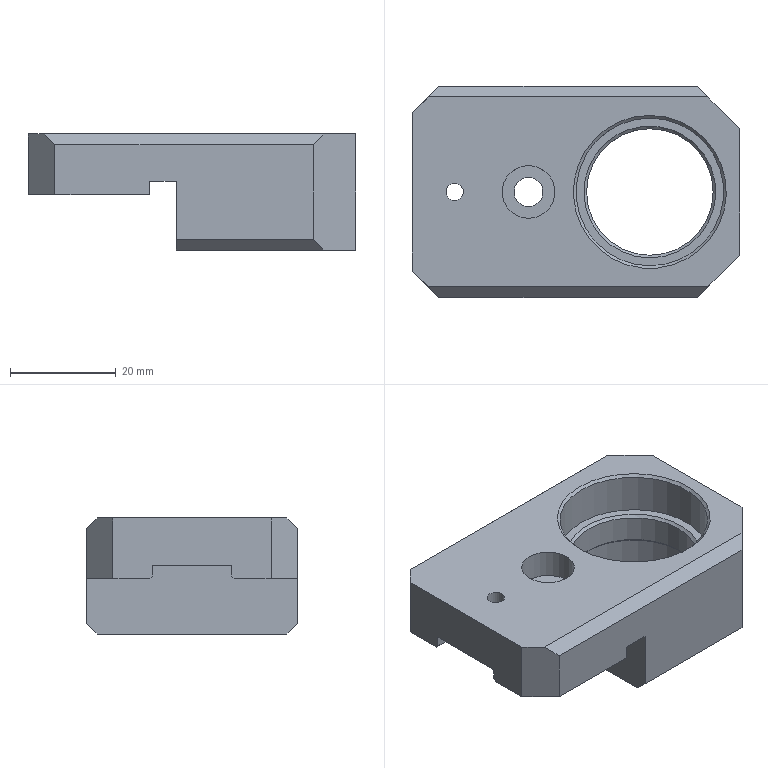NC program | NX | posted with a generic post | part box 62 x 40 x 22 mm
Whole program:
N10 G17 G21 G94 G90
(FLOOR_WALL , TOOL : D63)
N12 T01 M6
N14 G54
N16 G17 G0 G90 X-67.5 Y0. S6500 M3
N18 G43 Z30. H1
N20 Z3.
N22 G94 G1 Z0. F1500.
N24 X-64.5
N26 X64.5
N28 X67.5
N30 Z3.
N32 G0 Z30.
N34 M5
(DRILLING , TOOL : D8A45)
N36 T06 M6
N38 G54
N40 G17 G0 G90 X-9. Y0. S3500 M3
N42 G43 Z30. H6
N44 G94 G81 G98 Z-1. F250. R3.
N46 X14.
N48 X-23.
N50 G80
N52 G0 X-23. Y0. Z30.
N54 M5
(DRILLING_COPY , TOOL : 3.3ZT)
N56 T12 M6
N58 G54
N60 G17 G0 G90 X-23. Y0. S1500 M3
N62 G43 Z30. H12
N64 G94 G83 G98 Z-11.491 F150. Q2. R3.
N66 G80
N68 G0 X-23. Y0. Z30.
N70 M5
(DRILLING_1 , TOOL : 5.5ZT)
N72 T22 M6
N74 G54
N76 G17 G0 G90 X-9. Y0. S2000 M3
N78 G43 Z30. H22
N80 G94 G83 G98 Z-12.152 F200. Q3. R3.
N82 G80
N84 G0 X-9. Y0. Z30.
N86 M5
(ZLEVEL_PROFILE , TOOL : D10)
N88 T04 M6
N90 G54
N92 G17 G0 G90 X36.1 Y-8.145 S7000 M3
N94 G43 Z30. H4
N96 Z1.5
N98 G94 G1 Y-12. Z1.298 F1000.
N100 Y-12.554 Z1.269
N102 X35.74 Y-13.963 Z1.193
N104 X34.998 Y-15.215 Z1.116
N106 X26.215 Y-23.998 Z0.465
N108 X24.963 Y-24.74 Z0.389
N110 X23.554 Y-25.1 Z0.313
N112 X-1.5 Z-1.
N114 X-26. F3000.
N116 G2 X-29.606 Y-23.606 R5.1
N118 G1 X-34.606 Y-18.606
N120 G2 X-36.1 Y-15. R5.1
N122 G1 Y15.
N124 G2 X-34.606 Y18.606 R5.1
N126 G1 X-29.606 Y23.606
N128 G2 X-26. Y25.1 R5.1
N130 G1 X23.
N132 G2 X26.606 Y23.606 R5.1
N134 G1 X34.606 Y15.606
N136 G2 X36.1 Y12. R5.1
N138 G1 Y-12.
N140 G2 X34.606 Y-15.606 R5.1
N142 G1 X26.606 Y-23.606
N144 G2 X23. Y-25.1 R5.1
N146 G1 X-1.5
N148 X-25.5 Z-1.419
N150 X-25.887 Z-1.426
N152 X-26.274 Y-25.093 Z-1.432
N154 X-26.659 Y-25.057 Z-1.439
N156 X-27.041 Y-24.993 Z-1.446
N158 X-27.416 Y-24.899 Z-1.453
N160 X-27.784 Y-24.778 Z-1.459
N162 X-28.141 Y-24.629 Z-1.466
N164 X-28.486 Y-24.453 Z-1.473
N166 X-28.816 Y-24.252 Z-1.48
N168 X-29.131 Y-24.026 Z-1.486
N170 X-29.427 Y-23.777 Z-1.493
N172 X-29.705 Y-23.508 Z-1.5
N174 X-34.358 Y-18.854 Z-1.615
N176 X-34.632 Y-18.581 Z-1.622
N178 X-34.893 Y-18.295 Z-1.628
N180 X-35.131 Y-17.99 Z-1.635
N182 X-35.346 Y-17.668 Z-1.642
N184 X-35.536 Y-17.331 Z-1.649
N186 X-35.7 Y-16.98 Z-1.655
N188 X-35.836 Y-16.618 Z-1.662
N190 X-35.945 Y-16.247 Z-1.669
N192 X-36.026 Y-15.868 Z-1.676
N194 X-36.077 Y-15.485 Z-1.682
N196 X-36.099 Y-15.099 Z-1.689
N198 X-36.1 Y-14.711 Z-1.696
N200 Y-14.324 Z-1.703
N202 Y2.708 Z-2.
N204 Y15.
N206 G2 X-34.606 Y18.606 R5.1
N208 G1 X-29.606 Y23.606
N210 G2 X-26. Y25.1 R5.1
N212 G1 X23.
N214 G2 X26.606 Y23.606 R5.1
N216 G1 X34.606 Y15.606
N218 G2 X36.1 Y12. R5.1
N220 G1 Y-12.
N222 G2 X34.606 Y-15.606 R5.1
N224 G1 X26.606 Y-23.606
N226 G2 X23. Y-25.1 R5.1
N228 G1 X-1.5
N230 X-25.5 Z-2.419
N232 X-25.887 Z-2.426
N234 X-26.274 Y-25.093 Z-2.432
N236 X-26.659 Y-25.057 Z-2.439
N238 X-27.041 Y-24.993 Z-2.446
N240 X-27.416 Y-24.899 Z-2.453
N242 X-27.784 Y-24.778 Z-2.459
N244 X-28.141 Y-24.629 Z-2.466
N246 X-28.486 Y-24.453 Z-2.473
N248 X-28.816 Y-24.252 Z-2.48
N250 X-29.131 Y-24.026 Z-2.486
N252 X-29.427 Y-23.777 Z-2.493
N254 X-29.705 Y-23.508 Z-2.5
N256 X-34.358 Y-18.854 Z-2.615
N258 X-34.632 Y-18.581 Z-2.622
N260 X-34.893 Y-18.295 Z-2.628
N262 X-35.131 Y-17.99 Z-2.635
N264 X-35.346 Y-17.668 Z-2.642
N266 X-35.536 Y-17.331 Z-2.649
N268 X-35.7 Y-16.98 Z-2.655
N270 X-35.836 Y-16.618 Z-2.662
N272 X-35.945 Y-16.247 Z-2.669
N274 X-36.026 Y-15.868 Z-2.676
N276 X-36.077 Y-15.485 Z-2.682
N278 X-36.099 Y-15.099 Z-2.689
N280 X-36.1 Y-14.711 Z-2.696
N282 Y-14.324 Z-2.703
N284 Y2.708 Z-3.
N286 Y15.
N288 G2 X-34.606 Y18.606 R5.1
N290 G1 X-29.606 Y23.606
N292 G2 X-26. Y25.1 R5.1
N294 G1 X23.
N296 G2 X26.606 Y23.606 R5.1
N298 G1 X34.606 Y15.606
N300 G2 X36.1 Y12. R5.1
N302 G1 Y-12.
N304 G2 X34.606 Y-15.606 R5.1
N306 G1 X26.606 Y-23.606
N308 G2 X23. Y-25.1 R5.1
N310 G1 X-1.5
N312 X-25.5 Z-3.419
N314 X-25.887 Z-3.426
N316 X-26.274 Y-25.093 Z-3.432
N318 X-26.659 Y-25.057 Z-3.439
N320 X-27.041 Y-24.993 Z-3.446
N322 X-27.416 Y-24.899 Z-3.453
N324 X-27.784 Y-24.778 Z-3.459
N326 X-28.141 Y-24.629 Z-3.466
N328 X-28.486 Y-24.453 Z-3.473
N330 X-28.816 Y-24.252 Z-3.48
N332 X-29.131 Y-24.026 Z-3.486
N334 X-29.427 Y-23.777 Z-3.493
N336 X-29.705 Y-23.508 Z-3.5
N338 X-34.358 Y-18.854 Z-3.615
N340 X-34.632 Y-18.581 Z-3.622
N342 X-34.893 Y-18.295 Z-3.628
N344 X-35.131 Y-17.99 Z-3.635
N346 X-35.346 Y-17.668 Z-3.642
N348 X-35.536 Y-17.331 Z-3.649
N350 X-35.7 Y-16.98 Z-3.655
N352 X-35.836 Y-16.618 Z-3.662
N354 X-35.945 Y-16.247 Z-3.669
N356 X-36.026 Y-15.868 Z-3.676
N358 X-36.077 Y-15.485 Z-3.682
N360 X-36.099 Y-15.099 Z-3.689
N362 X-36.1 Y-14.711 Z-3.696
N364 Y-14.324 Z-3.703
N366 Y2.708 Z-4.
N368 Y15.
N370 G2 X-34.606 Y18.606 R5.1
N372 G1 X-29.606 Y23.606
N374 G2 X-26. Y25.1 R5.1
N376 G1 X23.
N378 G2 X26.606 Y23.606 R5.1
N380 G1 X34.606 Y15.606
N382 G2 X36.1 Y12. R5.1
N384 G1 Y-12.
N386 G2 X34.606 Y-15.606 R5.1
N388 G1 X26.606 Y-23.606
N390 G2 X23. Y-25.1 R5.1
N392 G1 X-1.5
N394 X-25.5 Z-4.419
N396 X-25.887 Z-4.426
N398 X-26.274 Y-25.093 Z-4.432
N400 X-26.659 Y-25.057 Z-4.439
N402 X-27.041 Y-24.993 Z-4.446
N404 X-27.416 Y-24.899 Z-4.453
N406 X-27.784 Y-24.778 Z-4.459
N408 X-28.141 Y-24.629 Z-4.466
N410 X-28.486 Y-24.453 Z-4.473
N412 X-28.816 Y-24.252 Z-4.48
N414 X-29.131 Y-24.026 Z-4.486
N416 X-29.427 Y-23.777 Z-4.493
N418 X-29.705 Y-23.508 Z-4.5
N420 X-34.358 Y-18.854 Z-4.615
N422 X-34.632 Y-18.581 Z-4.622
N424 X-34.893 Y-18.295 Z-4.628
N426 X-35.131 Y-17.99 Z-4.635
N428 X-35.346 Y-17.668 Z-4.642
N430 X-35.536 Y-17.331 Z-4.649
N432 X-35.7 Y-16.98 Z-4.655
N434 X-35.836 Y-16.618 Z-4.662
N436 X-35.945 Y-16.247 Z-4.669
N438 X-36.026 Y-15.868 Z-4.676
N440 X-36.077 Y-15.485 Z-4.682
N442 X-36.099 Y-15.099 Z-4.689
N444 X-36.1 Y-14.711 Z-4.696
N446 Y-14.324 Z-4.703
N448 Y2.708 Z-5.
N450 Y15.
N452 G2 X-34.606 Y18.606 R5.1
N454 G1 X-29.606 Y23.606
N456 G2 X-26. Y25.1 R5.1
N458 G1 X23.
N460 G2 X26.606 Y23.606 R5.1
N462 G1 X34.606 Y15.606
N464 G2 X36.1 Y12. R5.1
N466 G1 Y-12.
N468 G2 X34.606 Y-15.606 R5.1
N470 G1 X26.606 Y-23.606
N472 G2 X23. Y-25.1 R5.1
N474 G1 X-1.5
N476 X-25.5 Z-5.419
N478 X-25.887 Z-5.426
N480 X-26.274 Y-25.093 Z-5.432
N482 X-26.659 Y-25.057 Z-5.439
N484 X-27.041 Y-24.993 Z-5.446
N486 X-27.416 Y-24.899 Z-5.453
N488 X-27.784 Y-24.778 Z-5.459
N490 X-28.141 Y-24.629 Z-5.466
N492 X-28.486 Y-24.453 Z-5.473
N494 X-28.816 Y-24.252 Z-5.48
N496 X-29.131 Y-24.026 Z-5.486
N498 X-29.427 Y-23.777 Z-5.493
N500 X-29.705 Y-23.508 Z-5.5
N502 X-34.358 Y-18.854 Z-5.615
N504 X-34.632 Y-18.581 Z-5.622
N506 X-34.893 Y-18.295 Z-5.628
N508 X-35.131 Y-17.99 Z-5.635
N510 X-35.346 Y-17.668 Z-5.642
N512 X-35.536 Y-17.331 Z-5.649
N514 X-35.7 Y-16.98 Z-5.655
N516 X-35.836 Y-16.618 Z-5.662
N518 X-35.945 Y-16.247 Z-5.669
N520 X-36.026 Y-15.868 Z-5.676
N522 X-36.077 Y-15.485 Z-5.682
N524 X-36.099 Y-15.099 Z-5.689
N526 X-36.1 Y-14.711 Z-5.696
N528 Y-14.324 Z-5.703
N530 Y2.708 Z-6.
N532 Y15.
N534 G2 X-34.606 Y18.606 R5.1
N536 G1 X-29.606 Y23.606
N538 G2 X-26. Y25.1 R5.1
N540 G1 X23.
N542 G2 X26.606 Y23.606 R5.1
N544 G1 X34.606 Y15.606
N546 G2 X36.1 Y12. R5.1
N548 G1 Y-12.
N550 G2 X34.606 Y-15.606 R5.1
N552 G1 X26.606 Y-23.606
N554 G2 X23. Y-25.1 R5.1
N556 G1 X-1.5
N558 X-25.5 Z-6.419
N560 X-25.887 Z-6.426
N562 X-26.274 Y-25.093 Z-6.432
N564 X-26.659 Y-25.057 Z-6.439
N566 X-27.041 Y-24.993 Z-6.446
N568 X-27.416 Y-24.899 Z-6.453
N570 X-27.784 Y-24.778 Z-6.459
N572 X-28.141 Y-24.629 Z-6.466
N574 X-28.486 Y-24.453 Z-6.473
N576 X-28.816 Y-24.252 Z-6.48
N578 X-29.131 Y-24.026 Z-6.486
N580 X-29.427 Y-23.777 Z-6.493
N582 X-29.705 Y-23.508 Z-6.5
N584 X-34.358 Y-18.854 Z-6.615
N586 X-34.632 Y-18.581 Z-6.622
N588 X-34.893 Y-18.295 Z-6.628
N590 X-35.131 Y-17.99 Z-6.635
N592 X-35.346 Y-17.668 Z-6.642
N594 X-35.536 Y-17.331 Z-6.649
N596 X-35.7 Y-16.98 Z-6.655
N598 X-35.836 Y-16.618 Z-6.662
N600 X-35.945 Y-16.247 Z-6.669
N602 X-36.026 Y-15.868 Z-6.676
N604 X-36.077 Y-15.485 Z-6.682
N606 X-36.099 Y-15.099 Z-6.689
N608 X-36.1 Y-14.711 Z-6.696
N610 Y-14.324 Z-6.703
N612 Y2.708 Z-7.
N614 Y15.
N616 G2 X-34.606 Y18.606 R5.1
N618 G1 X-29.606 Y23.606
N620 G2 X-26. Y25.1 R5.1
N622 G1 X23.
N624 G2 X26.606 Y23.606 R5.1
N626 G1 X34.606 Y15.606
N628 G2 X36.1 Y12. R5.1
N630 G1 Y-12.
N632 G2 X34.606 Y-15.606 R5.1
N634 G1 X26.606 Y-23.606
N636 G2 X23. Y-25.1 R5.1
N638 G1 X-1.5
N640 X-25.5 Z-7.419
N642 X-25.887 Z-7.426
N644 X-26.274 Y-25.093 Z-7.432
N646 X-26.659 Y-25.057 Z-7.439
N648 X-27.041 Y-24.993 Z-7.446
N650 X-27.416 Y-24.899 Z-7.453
N652 X-27.784 Y-24.778 Z-7.459
N654 X-28.141 Y-24.629 Z-7.466
N656 X-28.486 Y-24.453 Z-7.473
N658 X-28.816 Y-24.252 Z-7.48
N660 X-29.131 Y-24.026 Z-7.486
N662 X-29.427 Y-23.777 Z-7.493
N664 X-29.705 Y-23.508 Z-7.5
N666 X-34.358 Y-18.854 Z-7.615
N668 X-34.632 Y-18.581 Z-7.622
N670 X-34.893 Y-18.295 Z-7.628
N672 X-35.131 Y-17.99 Z-7.635
N674 X-35.346 Y-17.668 Z-7.642
N676 X-35.536 Y-17.331 Z-7.649
N678 X-35.7 Y-16.98 Z-7.655
N680 X-35.836 Y-16.618 Z-7.662
N682 X-35.945 Y-16.247 Z-7.669
N684 X-36.026 Y-15.868 Z-7.676
N686 X-36.077 Y-15.485 Z-7.682
N688 X-36.099 Y-15.099 Z-7.689
N690 X-36.1 Y-14.711 Z-7.696
N692 Y-14.324 Z-7.703
N694 Y2.708 Z-8.
N696 Y15.
N698 G2 X-34.606 Y18.606 R5.1
N700 G1 X-29.606 Y23.606
N702 G2 X-26. Y25.1 R5.1
N704 G1 X23.
N706 G2 X26.606 Y23.606 R5.1
N708 G1 X34.606 Y15.606
N710 G2 X36.1 Y12. R5.1
N712 G1 Y-12.
N714 G2 X34.606 Y-15.606 R5.1
N716 G1 X26.606 Y-23.606
N718 G2 X23. Y-25.1 R5.1
N720 G1 X-1.5
N722 X-25.5 Z-8.419
N724 X-25.887 Z-8.426
N726 X-26.274 Y-25.093 Z-8.432
N728 X-26.659 Y-25.057 Z-8.439
N730 X-27.041 Y-24.993 Z-8.446
N732 X-27.416 Y-24.899 Z-8.453
N734 X-27.784 Y-24.778 Z-8.459
N736 X-28.141 Y-24.629 Z-8.466
N738 X-28.486 Y-24.453 Z-8.473
N740 X-28.816 Y-24.252 Z-8.48
N742 X-29.131 Y-24.026 Z-8.486
N744 X-29.427 Y-23.777 Z-8.493
N746 X-29.705 Y-23.508 Z-8.5
N748 X-34.358 Y-18.854 Z-8.615
N750 X-34.632 Y-18.581 Z-8.622
N752 X-34.893 Y-18.295 Z-8.628
N754 X-35.131 Y-17.99 Z-8.635
N756 X-35.346 Y-17.668 Z-8.642
N758 X-35.536 Y-17.331 Z-8.649
N760 X-35.7 Y-16.98 Z-8.655
N762 X-35.836 Y-16.618 Z-8.662
N764 X-35.945 Y-16.247 Z-8.669
N766 X-36.026 Y-15.868 Z-8.676
N768 X-36.077 Y-15.485 Z-8.682
N770 X-36.099 Y-15.099 Z-8.689
N772 X-36.1 Y-14.711 Z-8.696
N774 Y-14.324 Z-8.703
N776 Y2.708 Z-9.
N778 Y15.
N780 G2 X-34.606 Y18.606 R5.1
N782 G1 X-29.606 Y23.606
N784 G2 X-26. Y25.1 R5.1
N786 G1 X23.
N788 G2 X26.606 Y23.606 R5.1
N790 G1 X34.606 Y15.606
N792 G2 X36.1 Y12. R5.1
N794 G1 Y-12.
N796 G2 X34.606 Y-15.606 R5.1
N798 G1 X26.606 Y-23.606
N800 G2 X23. Y-25.1 R5.1
N802 G1 X-1.5
N804 X-25.5 Z-9.419
N806 X-25.887 Z-9.426
N808 X-26.274 Y-25.093 Z-9.432
N810 X-26.659 Y-25.057 Z-9.439
N812 X-27.041 Y-24.993 Z-9.446
N814 X-27.416 Y-24.899 Z-9.453
N816 X-27.784 Y-24.778 Z-9.459
N818 X-28.141 Y-24.629 Z-9.466
N820 X-28.486 Y-24.453 Z-9.473
N822 X-28.816 Y-24.252 Z-9.48
N824 X-29.131 Y-24.026 Z-9.486
N826 X-29.427 Y-23.777 Z-9.493
N828 X-29.705 Y-23.508 Z-9.5
N830 X-34.358 Y-18.854 Z-9.615
N832 X-34.632 Y-18.581 Z-9.622
N834 X-34.893 Y-18.295 Z-9.628
N836 X-35.131 Y-17.99 Z-9.635
N838 X-35.346 Y-17.668 Z-9.642
N840 X-35.536 Y-17.331 Z-9.649
N842 X-35.7 Y-16.98 Z-9.655
N844 X-35.836 Y-16.618 Z-9.662
N846 X-35.945 Y-16.247 Z-9.669
N848 X-36.026 Y-15.868 Z-9.676
N850 X-36.077 Y-15.485 Z-9.682
N852 X-36.099 Y-15.099 Z-9.689
N854 X-36.1 Y-14.711 Z-9.696
N856 Y-14.324 Z-9.703
N858 Y2.708 Z-10.
N860 Y15.
N862 G2 X-34.606 Y18.606 R5.1
N864 G1 X-29.606 Y23.606
N866 G2 X-26. Y25.1 R5.1
N868 G1 X23.
N870 G2 X26.606 Y23.606 R5.1
N872 G1 X34.606 Y15.606
N874 G2 X36.1 Y12. R5.1
N876 G1 Y-12.
N878 G2 X34.606 Y-15.606 R5.1
N880 G1 X26.606 Y-23.606
N882 G2 X23. Y-25.1 R5.1
N884 G1 X-1.5
N886 X-25.5 Z-10.419
N888 X-25.887 Z-10.426
N890 X-26.274 Y-25.093 Z-10.432
N892 X-26.659 Y-25.057 Z-10.439
N894 X-27.041 Y-24.993 Z-10.446
N896 X-27.416 Y-24.899 Z-10.453
N898 X-27.784 Y-24.778 Z-10.459
N900 X-28.141 Y-24.629 Z-10.466
N902 X-28.486 Y-24.453 Z-10.473
N904 X-28.816 Y-24.252 Z-10.48
N906 X-29.131 Y-24.026 Z-10.486
N908 X-29.427 Y-23.777 Z-10.493
N910 X-29.705 Y-23.508 Z-10.5
N912 X-34.358 Y-18.854 Z-10.615
N914 X-34.632 Y-18.581 Z-10.622
N916 X-34.893 Y-18.295 Z-10.628
N918 X-35.131 Y-17.99 Z-10.635
N920 X-35.346 Y-17.668 Z-10.642
N922 X-35.536 Y-17.331 Z-10.649
N924 X-35.7 Y-16.98 Z-10.655
N926 X-35.836 Y-16.618 Z-10.662
N928 X-35.945 Y-16.247 Z-10.669
N930 X-36.026 Y-15.868 Z-10.676
N932 X-36.077 Y-15.485 Z-10.682
N934 X-36.099 Y-15.099 Z-10.689
N936 X-36.1 Y-14.711 Z-10.696
N938 Y-14.324 Z-10.703
N940 Y2.708 Z-11.
N942 Y15.
N944 G2 X-34.606 Y18.606 R5.1
N946 G1 X-29.606 Y23.606
N948 G2 X-26. Y25.1 R5.1
N950 G1 X23.
N952 G2 X26.606 Y23.606 R5.1
N954 G1 X34.606 Y15.606
N956 G2 X36.1 Y12. R5.1
N958 G1 Y-12.
N960 G2 X34.606 Y-15.606 R5.1
N962 G1 X26.606 Y-23.606
N964 G2 X23. Y-25.1 R5.1
N966 G1 X-1.5
N968 X-25.5 Z-11.419
N970 X-25.887 Z-11.426
N972 X-26.274 Y-25.093 Z-11.432
N974 X-26.659 Y-25.057 Z-11.439
N976 X-27.041 Y-24.993 Z-11.446
N978 X-27.416 Y-24.899 Z-11.453
N980 X-27.784 Y-24.778 Z-11.459
N982 X-28.141 Y-24.629 Z-11.466
N984 X-28.486 Y-24.453 Z-11.473
N986 X-28.816 Y-24.252 Z-11.48
N988 X-29.131 Y-24.026 Z-11.486
N990 X-29.427 Y-23.777 Z-11.493
N992 X-29.705 Y-23.508 Z-11.5
N994 X-34.358 Y-18.854 Z-11.615
N996 X-34.632 Y-18.581 Z-11.622
N998 X-34.893 Y-18.295 Z-11.628
N1000 X-35.131 Y-17.99 Z-11.635
N1002 X-35.346 Y-17.668 Z-11.642
N1004 X-35.536 Y-17.331 Z-11.649
N1006 X-35.7 Y-16.98 Z-11.655
N1008 X-35.836 Y-16.618 Z-11.662
N1010 X-35.945 Y-16.247 Z-11.669
N1012 X-36.026 Y-15.868 Z-11.676
N1014 X-36.077 Y-15.485 Z-11.682
N1016 X-36.099 Y-15.099 Z-11.689
N1018 X-36.1 Y-14.711 Z-11.696
N1020 Y-14.324 Z-11.703
N1022 Y2.708 Z-12.
N1024 Y15.
N1026 G2 X-34.606 Y18.606 R5.1
N1028 G1 X-29.606 Y23.606
N1030 G2 X-26. Y25.1 R5.1
N1032 G1 X23.
N1034 G2 X26.606 Y23.606 R5.1
N1036 G1 X34.606 Y15.606
N1038 G2 X36.1 Y12. R5.1
N1040 G1 Y-12.
N1042 G2 X34.606 Y-15.606 R5.1
N1044 G1 X26.606 Y-23.606
N1046 G2 X23. Y-25.1 R5.1
N1048 G1 X-1.5
N1050 X-25.5 Z-12.419
N1052 X-25.887 Z-12.426
N1054 X-26.274 Y-25.093 Z-12.432
N1056 X-26.659 Y-25.057 Z-12.439
N1058 X-27.041 Y-24.993 Z-12.446
N1060 X-27.416 Y-24.899 Z-12.453
N1062 X-27.784 Y-24.778 Z-12.459
N1064 X-28.141 Y-24.629 Z-12.466
N1066 X-28.486 Y-24.453 Z-12.473
N1068 X-28.816 Y-24.252 Z-12.48
N1070 X-29.131 Y-24.026 Z-12.486
N1072 X-29.427 Y-23.777 Z-12.493
N1074 X-29.705 Y-23.508 Z-12.5
N1076 X-34.358 Y-18.854 Z-12.615
N1078 X-34.632 Y-18.581 Z-12.622
N1080 X-34.893 Y-18.295 Z-12.628
N1082 X-35.131 Y-17.99 Z-12.635
N1084 X-35.346 Y-17.668 Z-12.642
N1086 X-35.536 Y-17.331 Z-12.649
N1088 X-35.7 Y-16.98 Z-12.655
N1090 X-35.836 Y-16.618 Z-12.662
N1092 X-35.945 Y-16.247 Z-12.669
N1094 X-36.026 Y-15.868 Z-12.676
N1096 X-36.077 Y-15.485 Z-12.682
N1098 X-36.099 Y-15.099 Z-12.689
N1100 X-36.1 Y-14.711 Z-12.696
N1102 Y-14.324 Z-12.703
N1104 Y2.708 Z-13.
N1106 Y15.
N1108 G2 X-34.606 Y18.606 R5.1
N1110 G1 X-29.606 Y23.606
N1112 G2 X-26. Y25.1 R5.1
N1114 G1 X23.
N1116 G2 X26.606 Y23.606 R5.1
N1118 G1 X34.606 Y15.606
N1120 G2 X36.1 Y12. R5.1
N1122 G1 Y-12.
N1124 G2 X34.606 Y-15.606 R5.1
N1126 G1 X26.606 Y-23.606
N1128 G2 X23. Y-25.1 R5.1
N1130 G1 X-1.5
N1132 X-25.5 Z-13.419
N1134 X-25.887 Z-13.426
N1136 X-26.274 Y-25.093 Z-13.432
N1138 X-26.659 Y-25.057 Z-13.439
N1140 X-27.041 Y-24.993 Z-13.446
N1142 X-27.416 Y-24.899 Z-13.453
N1144 X-27.784 Y-24.778 Z-13.459
N1146 X-28.141 Y-24.629 Z-13.466
N1148 X-28.486 Y-24.453 Z-13.473
N1150 X-28.816 Y-24.252 Z-13.48
N1152 X-29.131 Y-24.026 Z-13.486
N1154 X-29.427 Y-23.777 Z-13.493
N1156 X-29.705 Y-23.508 Z-13.5
N1158 X-34.358 Y-18.854 Z-13.615
N1160 X-34.632 Y-18.581 Z-13.622
N1162 X-34.893 Y-18.295 Z-13.628
N1164 X-35.131 Y-17.99 Z-13.635
N1166 X-35.346 Y-17.668 Z-13.642
N1168 X-35.536 Y-17.331 Z-13.649
N1170 X-35.7 Y-16.98 Z-13.655
N1172 X-35.836 Y-16.618 Z-13.662
N1174 X-35.945 Y-16.247 Z-13.669
N1176 X-36.026 Y-15.868 Z-13.676
N1178 X-36.077 Y-15.485 Z-13.682
N1180 X-36.099 Y-15.099 Z-13.689
N1182 X-36.1 Y-14.711 Z-13.696
N1184 Y-14.324 Z-13.703
N1186 Y2.708 Z-14.
N1188 Y15.
N1190 G2 X-34.606 Y18.606 R5.1
N1192 G1 X-29.606 Y23.606
N1194 G2 X-26. Y25.1 R5.1
N1196 G1 X23.
N1198 G2 X26.606 Y23.606 R5.1
N1200 G1 X34.606 Y15.606
N1202 G2 X36.1 Y12. R5.1
N1204 G1 Y-12.
N1206 G2 X34.606 Y-15.606 R5.1
N1208 G1 X26.606 Y-23.606
N1210 G2 X23. Y-25.1 R5.1
N1212 G1 X-1.5
N1214 X-25.5 Z-14.419
N1216 X-25.887 Z-14.426
N1218 X-26.274 Y-25.093 Z-14.432
N1220 X-26.659 Y-25.057 Z-14.439
N1222 X-27.041 Y-24.993 Z-14.446
N1224 X-27.416 Y-24.899 Z-14.453
N1226 X-27.784 Y-24.778 Z-14.459
N1228 X-28.141 Y-24.629 Z-14.466
N1230 X-28.486 Y-24.453 Z-14.473
N1232 X-28.816 Y-24.252 Z-14.48
N1234 X-29.131 Y-24.026 Z-14.486
N1236 X-29.427 Y-23.777 Z-14.493
N1238 X-29.705 Y-23.508 Z-14.5
N1240 X-34.358 Y-18.854 Z-14.615
N1242 X-34.632 Y-18.581 Z-14.622
N1244 X-34.893 Y-18.295 Z-14.628
N1246 X-35.131 Y-17.99 Z-14.635
N1248 X-35.346 Y-17.668 Z-14.642
N1250 X-35.536 Y-17.331 Z-14.649
N1252 X-35.7 Y-16.98 Z-14.655
N1254 X-35.836 Y-16.618 Z-14.662
N1256 X-35.945 Y-16.247 Z-14.669
N1258 X-36.026 Y-15.868 Z-14.676
N1260 X-36.077 Y-15.485 Z-14.682
N1262 X-36.099 Y-15.099 Z-14.689
N1264 X-36.1 Y-14.711 Z-14.696
N1266 Y-14.324 Z-14.703
N1268 Y2.708 Z-15.
N1270 Y15.
N1272 G2 X-34.606 Y18.606 R5.1
N1274 G1 X-29.606 Y23.606
N1276 G2 X-26. Y25.1 R5.1
N1278 G1 X23.
N1280 G2 X26.606 Y23.606 R5.1
N1282 G1 X34.606 Y15.606
N1284 G2 X36.1 Y12. R5.1
N1286 G1 Y-12.
N1288 G2 X34.606 Y-15.606 R5.1
N1290 G1 X26.606 Y-23.606
N1292 G2 X23. Y-25.1 R5.1
N1294 G1 X-1.5
N1296 X-25.5 Z-15.419
N1298 X-25.887 Z-15.426
N1300 X-26.274 Y-25.093 Z-15.432
N1302 X-26.659 Y-25.057 Z-15.439
N1304 X-27.041 Y-24.993 Z-15.446
N1306 X-27.416 Y-24.899 Z-15.453
N1308 X-27.784 Y-24.778 Z-15.459
N1310 X-28.141 Y-24.629 Z-15.466
N1312 X-28.486 Y-24.453 Z-15.473
N1314 X-28.816 Y-24.252 Z-15.48
N1316 X-29.131 Y-24.026 Z-15.486
N1318 X-29.427 Y-23.777 Z-15.493
N1320 X-29.705 Y-23.508 Z-15.5
N1322 X-34.358 Y-18.854 Z-15.615
N1324 X-34.632 Y-18.581 Z-15.622
N1326 X-34.893 Y-18.295 Z-15.628
N1328 X-35.131 Y-17.99 Z-15.635
N1330 X-35.346 Y-17.668 Z-15.642
N1332 X-35.536 Y-17.331 Z-15.649
N1334 X-35.7 Y-16.98 Z-15.655
N1336 X-35.836 Y-16.618 Z-15.662
N1338 X-35.945 Y-16.247 Z-15.669
N1340 X-36.026 Y-15.868 Z-15.676
N1342 X-36.077 Y-15.485 Z-15.682
N1344 X-36.099 Y-15.099 Z-15.689
N1346 X-36.1 Y-14.711 Z-15.696
N1348 Y-14.324 Z-15.703
N1350 Y2.708 Z-16.
N1352 Y15.
N1354 G2 X-34.606 Y18.606 R5.1
N1356 G1 X-29.606 Y23.606
N1358 G2 X-26. Y25.1 R5.1
N1360 G1 X23.
N1362 G2 X26.606 Y23.606 R5.1
N1364 G1 X34.606 Y15.606
N1366 G2 X36.1 Y12. R5.1
N1368 G1 Y-12.
N1370 G2 X34.606 Y-15.606 R5.1
N1372 G1 X26.606 Y-23.606
N1374 G2 X23. Y-25.1 R5.1
N1376 G1 X-1.5
N1378 X-25.5 Z-16.419
N1380 X-25.887 Z-16.426
N1382 X-26.274 Y-25.093 Z-16.432
N1384 X-26.659 Y-25.057 Z-16.439
N1386 X-27.041 Y-24.993 Z-16.446
N1388 X-27.416 Y-24.899 Z-16.453
N1390 X-27.784 Y-24.778 Z-16.459
N1392 X-28.141 Y-24.629 Z-16.466
N1394 X-28.486 Y-24.453 Z-16.473
N1396 X-28.816 Y-24.252 Z-16.48
N1398 X-29.131 Y-24.026 Z-16.486
N1400 X-29.427 Y-23.777 Z-16.493
N1402 X-29.705 Y-23.508 Z-16.5
N1404 X-34.358 Y-18.854 Z-16.615
N1406 X-34.632 Y-18.581 Z-16.622
N1408 X-34.893 Y-18.295 Z-16.628
N1410 X-35.131 Y-17.99 Z-16.635
N1412 X-35.346 Y-17.668 Z-16.642
N1414 X-35.536 Y-17.331 Z-16.649
N1416 X-35.7 Y-16.98 Z-16.655
N1418 X-35.836 Y-16.618 Z-16.662
N1420 X-35.945 Y-16.247 Z-16.669
N1422 X-36.026 Y-15.868 Z-16.676
N1424 X-36.077 Y-15.485 Z-16.682
N1426 X-36.099 Y-15.099 Z-16.689
N1428 X-36.1 Y-14.711 Z-16.696
N1430 Y-14.324 Z-16.703
N1432 Y2.708 Z-17.
N1434 Y15.
N1436 G2 X-34.606 Y18.606 R5.1
N1438 G1 X-29.606 Y23.606
N1440 G2 X-26. Y25.1 R5.1
N1442 G1 X23.
N1444 G2 X26.606 Y23.606 R5.1
N1446 G1 X34.606 Y15.606
N1448 G2 X36.1 Y12. R5.1
N1450 G1 Y-12.
N1452 G2 X34.606 Y-15.606 R5.1
N1454 G1 X26.606 Y-23.606
N1456 G2 X23. Y-25.1 R5.1
N1458 G1 X-1.5
N1460 X-25.5 Z-17.419
N1462 X-25.887 Z-17.426
N1464 X-26.274 Y-25.093 Z-17.432
N1466 X-26.659 Y-25.057 Z-17.439
N1468 X-27.041 Y-24.993 Z-17.446
N1470 X-27.416 Y-24.899 Z-17.453
N1472 X-27.784 Y-24.778 Z-17.459
N1474 X-28.141 Y-24.629 Z-17.466
N1476 X-28.486 Y-24.453 Z-17.473
N1478 X-28.816 Y-24.252 Z-17.48
N1480 X-29.131 Y-24.026 Z-17.486
N1482 X-29.427 Y-23.777 Z-17.493
N1484 X-29.705 Y-23.508 Z-17.5
N1486 X-34.358 Y-18.854 Z-17.615
N1488 X-34.632 Y-18.581 Z-17.622
N1490 X-34.893 Y-18.295 Z-17.628
N1492 X-35.131 Y-17.99 Z-17.635
N1494 X-35.346 Y-17.668 Z-17.642
N1496 X-35.536 Y-17.331 Z-17.649
N1498 X-35.7 Y-16.98 Z-17.655
N1500 X-35.836 Y-16.618 Z-17.662
N1502 X-35.945 Y-16.247 Z-17.669
N1504 X-36.026 Y-15.868 Z-17.676
N1506 X-36.077 Y-15.485 Z-17.682
N1508 X-36.099 Y-15.099 Z-17.689
N1510 X-36.1 Y-14.711 Z-17.696
N1512 Y-14.324 Z-17.703
N1514 Y2.708 Z-18.
N1516 Y15.
N1518 G2 X-34.606 Y18.606 R5.1
N1520 G1 X-29.606 Y23.606
N1522 G2 X-26. Y25.1 R5.1
N1524 G1 X23.
N1526 G2 X26.606 Y23.606 R5.1
N1528 G1 X34.606 Y15.606
N1530 G2 X36.1 Y12. R5.1
N1532 G1 Y-12.
N1534 G2 X34.606 Y-15.606 R5.1
N1536 G1 X26.606 Y-23.606
N1538 G2 X23. Y-25.1 R5.1
N1540 G1 X-1.5
N1542 X-25.5 Z-18.419
N1544 X-25.887 Z-18.426
N1546 X-26.274 Y-25.093 Z-18.432
N1548 X-26.659 Y-25.057 Z-18.439
N1550 X-27.041 Y-24.993 Z-18.446
N1552 X-27.416 Y-24.899 Z-18.453
N1554 X-27.784 Y-24.778 Z-18.459
N1556 X-28.141 Y-24.629 Z-18.466
N1558 X-28.486 Y-24.453 Z-18.473
N1560 X-28.816 Y-24.252 Z-18.48
N1562 X-29.131 Y-24.026 Z-18.486
N1564 X-29.427 Y-23.777 Z-18.493
N1566 X-29.705 Y-23.508 Z-18.5
N1568 X-34.358 Y-18.854 Z-18.615
N1570 X-34.632 Y-18.581 Z-18.622
N1572 X-34.893 Y-18.295 Z-18.628
N1574 X-35.131 Y-17.99 Z-18.635
N1576 X-35.346 Y-17.668 Z-18.642
N1578 X-35.536 Y-17.331 Z-18.649
N1580 X-35.7 Y-16.98 Z-18.655
N1582 X-35.836 Y-16.618 Z-18.662
N1584 X-35.945 Y-16.247 Z-18.669
N1586 X-36.026 Y-15.868 Z-18.676
N1588 X-36.077 Y-15.485 Z-18.682
N1590 X-36.099 Y-15.099 Z-18.689
N1592 X-36.1 Y-14.711 Z-18.696
N1594 Y-14.324 Z-18.703
N1596 Y2.708 Z-19.
N1598 Y15.
N1600 G2 X-34.606 Y18.606 R5.1
N1602 G1 X-29.606 Y23.606
N1604 G2 X-26. Y25.1 R5.1
N1606 G1 X23.
N1608 G2 X26.606 Y23.606 R5.1
N1610 G1 X34.606 Y15.606
N1612 G2 X36.1 Y12. R5.1
N1614 G1 Y-12.
N1616 G2 X34.606 Y-15.606 R5.1
N1618 G1 X26.606 Y-23.606
N1620 G2 X23. Y-25.1 R5.1
N1622 G1 X-1.5
N1624 X-25.5 Z-19.419
N1626 X-25.887 Z-19.426
N1628 X-26.274 Y-25.093 Z-19.432
N1630 X-26.659 Y-25.057 Z-19.439
N1632 X-27.041 Y-24.993 Z-19.446
N1634 X-27.416 Y-24.899 Z-19.453
N1636 X-27.784 Y-24.778 Z-19.459
N1638 X-28.141 Y-24.629 Z-19.466
N1640 X-28.486 Y-24.453 Z-19.473
N1642 X-28.816 Y-24.252 Z-19.48
N1644 X-29.131 Y-24.026 Z-19.486
N1646 X-29.427 Y-23.777 Z-19.493
N1648 X-29.705 Y-23.508 Z-19.5
N1650 X-34.358 Y-18.854 Z-19.615
N1652 X-34.632 Y-18.581 Z-19.622
N1654 X-34.893 Y-18.295 Z-19.628
N1656 X-35.131 Y-17.99 Z-19.635
N1658 X-35.346 Y-17.668 Z-19.642
N1660 X-35.536 Y-17.331 Z-19.649
N1662 X-35.7 Y-16.98 Z-19.655
N1664 X-35.836 Y-16.618 Z-19.662
N1666 X-35.945 Y-16.247 Z-19.669
N1668 X-36.026 Y-15.868 Z-19.676
N1670 X-36.077 Y-15.485 Z-19.682
N1672 X-36.099 Y-15.099 Z-19.689
N1674 X-36.1 Y-14.711 Z-19.696
N1676 Y-14.324 Z-19.703
N1678 Y2.708 Z-20.
N1680 Y15.
N1682 G2 X-34.606 Y18.606 R5.1
N1684 G1 X-29.606 Y23.606
N1686 G2 X-26. Y25.1 R5.1
N1688 G1 X23.
N1690 G2 X26.606 Y23.606 R5.1
N1692 G1 X34.606 Y15.606
N1694 G2 X36.1 Y12. R5.1
N1696 G1 Y-12.
N1698 G2 X34.606 Y-15.606 R5.1
N1700 G1 X26.606 Y-23.606
N1702 G2 X23. Y-25.1 R5.1
N1704 G1 X-1.5
N1706 X-25.5 Z-20.419
N1708 X-25.887 Z-20.426
N1710 X-26.274 Y-25.093 Z-20.432
N1712 X-26.659 Y-25.057 Z-20.439
N1714 X-27.041 Y-24.993 Z-20.446
N1716 X-27.416 Y-24.899 Z-20.453
N1718 X-27.784 Y-24.778 Z-20.459
N1720 X-28.141 Y-24.629 Z-20.466
N1722 X-28.486 Y-24.453 Z-20.473
N1724 X-28.816 Y-24.252 Z-20.48
N1726 X-29.131 Y-24.026 Z-20.486
N1728 X-29.427 Y-23.777 Z-20.493
N1730 X-29.705 Y-23.508 Z-20.5
N1732 X-34.358 Y-18.854 Z-20.615
N1734 X-34.632 Y-18.581 Z-20.622
N1736 X-34.893 Y-18.295 Z-20.628
N1738 X-35.131 Y-17.99 Z-20.635
N1740 X-35.346 Y-17.668 Z-20.642
N1742 X-35.536 Y-17.331 Z-20.649
N1744 X-35.7 Y-16.98 Z-20.655
N1746 X-35.836 Y-16.618 Z-20.662
N1748 X-35.945 Y-16.247 Z-20.669
N1750 X-36.026 Y-15.868 Z-20.676
N1752 X-36.077 Y-15.485 Z-20.682
N1754 X-36.099 Y-15.099 Z-20.689
N1756 X-36.1 Y-14.711 Z-20.696
N1758 Y-14.324 Z-20.703
N1760 Y2.708 Z-21.
N1762 Y15.
N1764 G2 X-34.606 Y18.606 R5.1
N1766 G1 X-29.606 Y23.606
N1768 G2 X-26. Y25.1 R5.1
N1770 G1 X23.
N1772 G2 X26.606 Y23.606 R5.1
N1774 G1 X34.606 Y15.606
N1776 G2 X36.1 Y12. R5.1
N1778 G1 Y-12.
N1780 G2 X34.606 Y-15.606 R5.1
N1782 G1 X26.606 Y-23.606
N1784 G2 X23. Y-25.1 R5.1
N1786 G1 X-1.5
N1788 X-25.5 Z-21.419
N1790 X-25.887 Z-21.426
N1792 X-26.274 Y-25.093 Z-21.432
N1794 X-26.659 Y-25.057 Z-21.439
N1796 X-27.041 Y-24.993 Z-21.446
N1798 X-27.416 Y-24.899 Z-21.453
N1800 X-27.784 Y-24.778 Z-21.459
N1802 X-28.141 Y-24.629 Z-21.466
N1804 X-28.486 Y-24.453 Z-21.473
N1806 X-28.816 Y-24.252 Z-21.48
N1808 X-29.131 Y-24.026 Z-21.486
N1810 X-29.427 Y-23.777 Z-21.493
N1812 X-29.705 Y-23.508 Z-21.5
N1814 X-34.358 Y-18.854 Z-21.615
N1816 X-34.632 Y-18.581 Z-21.622
N1818 X-34.893 Y-18.295 Z-21.628
N1820 X-35.131 Y-17.99 Z-21.635
N1822 X-35.346 Y-17.668 Z-21.642
N1824 X-35.536 Y-17.331 Z-21.649
N1826 X-35.7 Y-16.98 Z-21.655
N1828 X-35.836 Y-16.618 Z-21.662
N1830 X-35.945 Y-16.247 Z-21.669
N1832 X-36.026 Y-15.868 Z-21.676
N1834 X-36.077 Y-15.485 Z-21.682
N1836 X-36.099 Y-15.099 Z-21.689
N1838 X-36.1 Y-14.711 Z-21.696
N1840 Y-14.324 Z-21.703
N1842 Y2.708 Z-22.
N1844 Y15.
N1846 G2 X-34.606 Y18.606 R5.1
N1848 G1 X-29.606 Y23.606
N1850 G2 X-26. Y25.1 R5.1
N1852 G1 X23.
N1854 G2 X26.606 Y23.606 R5.1
N1856 G1 X34.606 Y15.606
N1858 G2 X36.1 Y12. R5.1
N1860 G1 Y-12.
N1862 G2 X34.606 Y-15.606 R5.1
N1864 G1 X26.606 Y-23.606
N1866 G2 X23. Y-25.1 R5.1
N1868 G1 X-26.
N1870 G2 X-29.606 Y-23.606 R5.1
N1872 G1 X-34.606 Y-18.606
N1874 G2 X-36.1 Y-15. R5.1
N1876 G1 Y2.708
N1878 Z-20.5
N1880 G0 Z30.
(HOLE_MILLING , TOOL : D10)
N1882 X14. Y0.
N1884 Z0.5
N1886 G3 X16.225 Y-2.225 R2.225 F2000.
N1888 X18.45 Y0. R2.225
N1890 X18.45 Y0. Z-0.5 I-4.45 J0.
N1892 X18.45 Y0. Z-1.5 I-4.45 J0.
N1894 X18.45 Y0. Z-2.5 I-4.45 J0.
N1896 X18.45 Y0. Z-3.5 I-4.45 J0.
N1898 X18.45 Y0. Z-4.5 I-4.45 J0.
N1900 X18.45 Y0. Z-5.5 I-4.45 J0.
N1902 X18.45 Y0. Z-6.5 I-4.45 J0.
N1904 X18.45 Y0. Z-7.5 I-4.45 J0.
N1906 X9.55 Y0. Z-8. I-4.45 J0.
N1908 X14. Y-4.45 R4.45
N1910 X9.55 Y0. R-4.45
N1912 X11.775 Y-2.225 R2.225
N1914 X14. Y0. R2.225
N1916 G0 Z0.5
N1918 G3 X18.45 Y-4.45 R4.45
N1920 X22.9 Y0. R4.45
N1922 X22.9 Y0. Z-0.5 I-8.9 J0.
N1924 X22.9 Y0. Z-1.5 I-8.9 J0.
N1926 X22.9 Y0. Z-2.5 I-8.9 J0.
N1928 X22.9 Y0. Z-3.5 I-8.9 J0.
N1930 X22.9 Y0. Z-4.5 I-8.9 J0.
N1932 X22.9 Y0. Z-5.5 I-8.9 J0.
N1934 X22.9 Y0. Z-6.5 I-8.9 J0.
N1936 X22.9 Y0. Z-7.5 I-8.9 J0.
N1938 X5.1 Y0. Z-8. I-8.9 J0.
N1940 X14. Y-8.9 R8.9
N1942 X5.1 Y0. R-8.9
N1944 X9.55 Y-4.45 R4.45
N1946 X14. Y0. R4.45
N1948 G0 Z30.
(HOLE_MILLING_COPY , TOOL : D10)
N1950 Z-7.5
N1952 G3 X15.725 Y-1.725 R1.725
N1954 X17.45 Y0. R1.725
N1956 X17.45 Y0. Z-8.5 I-3.45 J0.
N1958 X17.45 Y0. Z-9.5 I-3.45 J0.
N1960 X17.45 Y0. Z-10.5 I-3.45 J0.
N1962 X17.45 Y0. Z-11.5 I-3.45 J0.
N1964 X17.45 Y0. Z-12.5 I-3.45 J0.
N1966 X17.45 Y0. Z-13.5 I-3.45 J0.
N1968 X17.45 Y0. Z-14.5 I-3.45 J0.
N1970 X17.45 Y0. Z-15.5 I-3.45 J0.
N1972 X17.45 Y0. Z-16.5 I-3.45 J0.
N1974 X17.45 Y0. Z-17.5 I-3.45 J0.
N1976 X17.45 Y0. Z-18.5 I-3.45 J0.
N1978 X17.45 Y0. Z-19.5 I-3.45 J0.
N1980 X17.45 Y0. Z-20.5 I-3.45 J0.
N1982 X17.45 Y0. Z-21.5 I-3.45 J0.
N1984 X10.55 Y0. Z-22. I-3.45 J0.
N1986 X14. Y-3.45 R3.45
N1988 X10.55 Y0. R-3.45
N1990 X12.275 Y-1.725 R1.725
N1992 X14. Y0. R1.725
N1994 G0 Z-7.5
N1996 G3 X17.45 Y-3.45 R3.45
N1998 X20.9 Y0. R3.45
N2000 X20.9 Y0. Z-8.5 I-6.9 J0.
N2002 X20.9 Y0. Z-9.5 I-6.9 J0.
N2004 X20.9 Y0. Z-10.5 I-6.9 J0.
N2006 X20.9 Y0. Z-11.5 I-6.9 J0.
N2008 X20.9 Y0. Z-12.5 I-6.9 J0.
N2010 X20.9 Y0. Z-13.5 I-6.9 J0.
N2012 X20.9 Y0. Z-14.5 I-6.9 J0.
N2014 X20.9 Y0. Z-15.5 I-6.9 J0.
N2016 X20.9 Y0. Z-16.5 I-6.9 J0.
N2018 X20.9 Y0. Z-17.5 I-6.9 J0.
N2020 X20.9 Y0. Z-18.5 I-6.9 J0.
N2022 X20.9 Y0. Z-19.5 I-6.9 J0.
N2024 X20.9 Y0. Z-20.5 I-6.9 J0.
N2026 X20.9 Y0. Z-21.5 I-6.9 J0.
N2028 X7.1 Y0. Z-22. I-6.9 J0.
N2030 X14. Y-6.9 R6.9
N2032 X7.1 Y0. R-6.9
N2034 X10.55 Y-3.45 R3.45
N2036 X14. Y0. R3.45
N2038 G0 Z30.
(ZLEVEL_PROFILE_COPY , TOOL : D10)
N2040 X18.598 Y-1.964
N2042 Z-11.
N2044 G1 X20.5 Y-0.866 F1000.
N2046 G3 X21. Y0. R1.
N2048 X14. Y7. R7.
N2050 X21. Y0. R-7.
N2052 X20.5 Y0.866 R1.
N2054 G1 X18.598 Y1.964
N2056 G0 Y-1.964 Z-22.
N2058 G1 X20.5 Y-0.866
N2060 G3 X21. Y0. R1.
N2062 X14. Y7. R7.
N2064 X21. Y0. R-7.
N2066 X20.5 Y0.866 R1.
N2068 G1 X18.598 Y1.964
N2070 G0 Z30.
N2072 X24.622 Y-26.809
N2074 Z-11.
N2076 G1 X23.866 Y-25.5
N2078 G3 X23. Y-25. R1.
N2080 G1 X-26.
N2082 G2 X-29.536 Y-23.536 R5.
N2084 G1 X-34.536 Y-18.536
N2086 G2 X-36. Y-15. R5.
N2088 G1 Y15.
N2090 G2 X-34.536 Y18.536 R5.
N2092 G1 X-29.536 Y23.536
N2094 G2 X-26. Y25. R5.
N2096 G1 X23.
N2098 G2 X26.536 Y23.536 R5.
N2100 G1 X34.536 Y15.536
N2102 G2 X36. Y12. R5.
N2104 G1 Y-12.
N2106 G2 X34.536 Y-15.536 R5.
N2108 G1 X26.536 Y-23.536
N2110 G2 X23. Y-25. R5.
N2112 G3 X22.134 Y-25.5 R1.
N2114 G1 X21.268 Y-27.
N2116 G0 X24.622 Y-26.809 Z-22.
N2118 G1 X23.866 Y-25.5
N2120 G3 X23. Y-25. R1.
N2122 G1 X-26.
N2124 G2 X-29.536 Y-23.536 R5.
N2126 G1 X-34.536 Y-18.536
N2128 G2 X-36. Y-15. R5.
N2130 G1 Y15.
N2132 G2 X-34.536 Y18.536 R5.
N2134 G1 X-29.536 Y23.536
N2136 G2 X-26. Y25. R5.
N2138 G1 X23.
N2140 G2 X26.536 Y23.536 R5.
N2142 G1 X34.536 Y15.536
N2144 G2 X36. Y12. R5.
N2146 G1 Y-12.
N2148 G2 X34.536 Y-15.536 R5.
N2150 G1 X26.536 Y-23.536
N2152 G2 X23. Y-25. R5.
N2154 G3 X22.134 Y-25.5 R1.
N2156 G1 X21.268 Y-27.
N2158 G0 Z30.
N2160 M5
(HOLE_MILLING_1 , TOOL : D6)
N2162 T02 M6
N2164 G54
N2166 G17 G0 G90 X-9. Y0. S7000 M3
N2168 G43 Z30. H2
N2170 Z0.5
N2172 G94 G3 X-8. Y-1. R1. F1400.
N2174 X-7. Y0. R1.
N2176 X-7. Y0. Z0. I-2. J0.
N2178 X-7. Y0. Z-0.5 I-2. J0.
N2180 X-7. Y0. Z-1. I-2. J0.
N2182 X-7. Y0. Z-1.5 I-2. J0.
N2184 X-7. Y0. Z-2. I-2. J0.
N2186 X-7. Y0. Z-2.5 I-2. J0.
N2188 X-7. Y0. Z-3. I-2. J0.
N2190 X-7. Y0. Z-3.5 I-2. J0.
N2192 X-7. Y0. Z-4. I-2. J0.
N2194 X-7. Y0. Z-4.5 I-2. J0.
N2196 X-7. Y0. Z-5. I-2. J0.
N2198 X-8.382 Y-1.902 Z-5.4 R-2.
N2200 X-7.098 Y0.618 R2.
N2202 X-8.382 Y-1.902 R-2.
N2204 X-7.74 Y-0.642 R1.
N2206 X-9. Y0. R1.
N2208 G0 Z30.
N2210 M5
(PLANAR_MILL , TOOL : D8A45)
N2212 T06 M6
N2214 G54
N2216 G17 G0 G90 X0.001 Y-22.5 S7000 M3
N2218 G43 Z30. H6
N2220 Z0.5
N2222 G94 G1 Z-1. F1250.
N2224 X-0.634 Y-21.4
N2226 G3 X-1.5 Y-20.9 R1.
N2228 G1 X-25.959
N2230 G2 X-26.666 Y-20.607 R1.
N2232 G1 X-28.636 Y-18.636
N2234 X-31.607 Y-15.666
N2236 G2 X-31.9 Y-14.959 R1.
N2238 G1 Y14.959
N2240 G2 X-31.607 Y15.666 R1.
N2242 G1 X-26.666 Y20.607
N2244 G2 X-25.959 Y20.9 R1.
N2246 G1 X22.959
N2248 G2 X23.666 Y20.607 R1.
N2250 G1 X31.607 Y12.666
N2252 G2 X31.9 Y11.959 R1.
N2254 G1 Y-11.959
N2256 G2 X31.607 Y-12.666 R1.
N2258 G1 X25.636 Y-18.636
N2260 X23.666 Y-20.607
N2262 G2 X22.959 Y-20.9 R1.
N2264 G1 X-1.5
N2266 G3 X-2.366 Y-21.4 R1.
N2268 G1 X-3.001 Y-22.5
N2270 Z0.5
N2272 G0 Z30.
N2274 X12.437 Y-11.393
N2276 Z0.5
N2278 G1 Z-1.
N2280 X13.134 Y-12.6
N2282 G3 X14. Y-13.1 R1.
N2284 X27.1 Y0. R13.1
N2286 X14. Y-13.1 R-13.1
N2288 X14.866 Y-12.6 R1.
N2290 G1 X15.563 Y-11.393
N2292 Z0.5
N2294 G0 Z30.
N2296 X-9.585 Y-2.431
N2298 Z0.5
N2300 G1 Z-1.
N2302 X-9.866 Y-3.6
N2304 G3 X-9. Y-4.1 R1.
N2306 X-4.9 Y0. R4.1
N2308 X-9. Y-4.1 R-4.1
N2310 X-8.134 Y-3.6 R1.
N2312 G1 X-8.415 Y-2.431
N2314 Z0.5
N2316 G0 Z30.
N2318 X-23.387 Y0.676
N2320 Z0.5
N2322 G1 X-23.75 Y0.214 Z0.343
N2324 Y-0.214 Z0.228
N2326 X-23.39 Y-0.676 Z0.071
N2328 X-22.811 Y-0.757 Z-0.086
N2330 X-22.439 Y-0.542 Z-0.201
N2332 X-22.22 Y0. Z-0.357
N2334 X-22.439 Y0.542 Z-0.514
N2336 X-22.811 Y0.757 Z-0.629
N2338 X-23.39 Y0.676 Z-0.786
N2340 X-23.75 Y0.214 Z-0.943
N2342 Y0. Z-1.
N2344 G3 X-23. Y-0.75 R0.75
N2346 X-23.75 Y0. R-0.75
N2348 X-23.5 Y-0.433 R0.5
N2350 G1 Z0.5
N2352 G0 Z30.
(PLANAR_MILL_COPY , TOOL : D8A45)
N2354 X-29.501 Y22.6
N2356 Z-1.
N2358 G1 Z-2.5
N2360 X-28.866 Y21.5
N2362 G3 X-28. Y21. R1.
N2364 G1 X25.
N2366 G3 X25.866 Y21.5 R1.
N2368 G1 X26.501 Y22.6
N2370 Z-1.
N2372 G0 Z30.
N2374 X-29.79
N2376 Z-1.
N2378 G1 Z-2.5
N2380 X-28.866 Y21.
N2382 G3 X-28. Y20.5 R1.
N2384 G1 X25.
N2386 G3 X25.866 Y21. R1.
N2388 G1 X26.79 Y22.6
N2390 Z-1.
N2392 G0 Z30.
N2394 X24.324 Y-1.256
N2396 Z-1.
N2398 G1 Z-2.5
N2400 X25. Y-0.866
N2402 G3 X25.5 Y0. R1.
N2404 X14. Y11.5 R11.5
N2406 X25.5 Y0. R-11.5
N2408 X25. Y0.866 R1.
N2410 G1 X25.5 Y-0.866
N2412 G3 X26. Y0. R1.
N2414 X14. Y12. R12.
N2416 X26. Y0. R-12.
N2418 X25.5 Y0.866 R1.
N2420 G1 X24.281 Y1.57
N2422 Z-1.
N2424 G0 Z30.
N2426 X26.501 Y-22.6
N2428 Z-1.
N2430 G1 Z-2.5
N2432 X25.866 Y-21.5
N2434 G3 X25. Y-21. R1.
N2436 G1 X-28.
N2438 G3 X-28.866 Y-21.5 R1.
N2440 G1 X-29.501 Y-22.6
N2442 Z-1.
N2444 G0 Z30.
N2446 X26.79
N2448 Z-1.
N2450 G1 Z-2.5
N2452 X25.866 Y-21.
N2454 G3 X25. Y-20.5 R1.
N2456 G1 X-28.
N2458 G3 X-28.866 Y-21. R1.
N2460 G1 X-29.79 Y-22.6
N2462 Z-1.
N2464 G0 Z30.
N2466 M5
(CUTTERCOMP4 , TOOL : D10)
N2468 T04 M6
N2470 G54
N2472 G17 G0 G90 X14. Y0. S7000 M3
N2474 G43 Z30. H4
N2476 Z0.5
N2478 G41 G94 G1 X19.233 Y-2.725 F1000. D4
N2480 G3 X22.95 Y0. R2.857
N2482 X22.95 Y0. Z-2.5 I-8.95 J0.
N2484 X22.95 Y0. Z-5.5 I-8.95 J0.
N2486 X18.475 Y-7.751 Z-8. R-8.95
N2488 X21.751 Y4.475 R8.95
N2490 X18.475 Y-7.751 R-8.95
N2492 X18.976 Y-3.169 R2.857
N2494 G40
N2496 G1 X14. Y0.
N2498 G0 Z30.
N2500 M5
N2502 M2